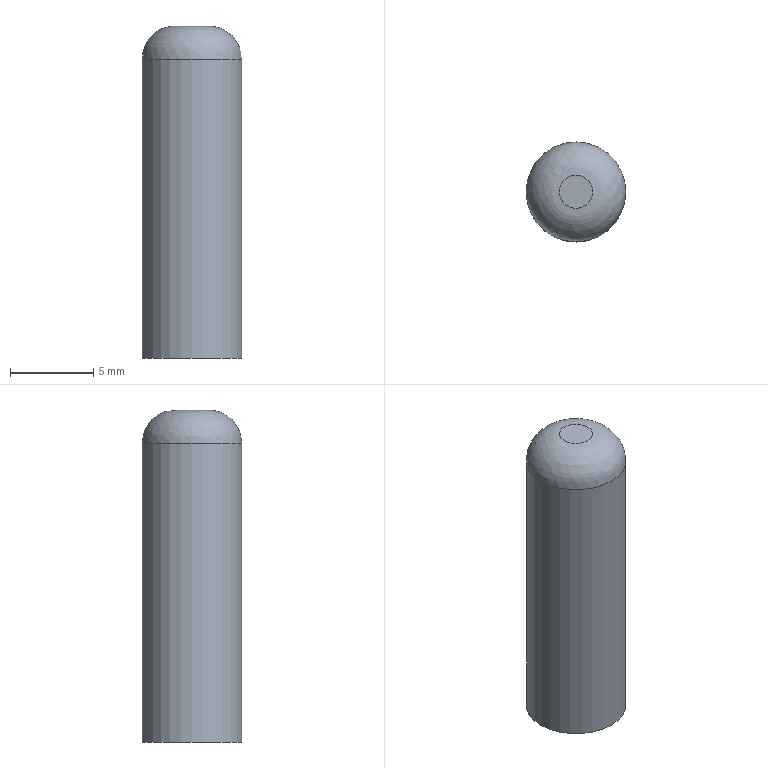Part | STEP file | SynoNew-0304-062 | 1 solid | 4 faces | box 6 x 6 x 20 mm | volume 551.703 mm3 | plane 2 | spline 1 | cylinder 1 | commonest cylinder face diameters 6 x1
STEP:
#1=CARTESIAN_POINT('',(1.,0.,20.));
#2=VERTEX_POINT('',#1);
#3=CARTESIAN_POINT('',(-1.,0.,20.));
#4=VERTEX_POINT('',#3);
#5=CARTESIAN_POINT('',(0.,0.,20.));
#6=DIRECTION('',(0.,0.,-1.));
#7=DIRECTION('',(-1.,0.,0.));
#8=AXIS2_PLACEMENT_3D('',#5,#6,#7);
#9=CIRCLE('',#8,1.);
#10=EDGE_CURVE('',#2,#4,#9,.T.);
#11=ORIENTED_EDGE('',*,*,#10,.T.);
#12=CARTESIAN_POINT('',(-3.,0.,18.));
#13=VERTEX_POINT('',#12);
#14=CARTESIAN_POINT('',(-1.,0.,18.));
#15=DIRECTION('',(0.,-1.,0.));
#16=DIRECTION('',(-1.,0.,0.));
#17=AXIS2_PLACEMENT_3D('',#14,#15,#16);
#18=CIRCLE('',#17,2.);
#19=EDGE_CURVE('',#4,#13,#18,.T.);
#20=ORIENTED_EDGE('',*,*,#19,.T.);
#21=CARTESIAN_POINT('',(3.,0.,18.));
#22=VERTEX_POINT('',#21);
#23=CARTESIAN_POINT('',(0.,0.,18.));
#24=DIRECTION('',(0.,0.,1.));
#25=DIRECTION('',(-1.,0.,0.));
#26=AXIS2_PLACEMENT_3D('',#23,#24,#25);
#27=CIRCLE('',#26,3.);
#28=EDGE_CURVE('',#13,#22,#27,.T.);
#29=ORIENTED_EDGE('',*,*,#28,.T.);
#30=CARTESIAN_POINT('',(0.,0.,18.));
#31=DIRECTION('',(0.,0.,1.));
#32=DIRECTION('',(-1.,0.,0.));
#33=AXIS2_PLACEMENT_3D('',#30,#31,#32);
#34=CIRCLE('',#33,3.);
#35=EDGE_CURVE('',#22,#13,#34,.T.);
#36=ORIENTED_EDGE('',*,*,#35,.T.);
#37=ORIENTED_EDGE('',*,*,#19,.F.);
#38=CARTESIAN_POINT('',(0.,0.,20.));
#39=DIRECTION('',(0.,0.,-1.));
#40=DIRECTION('',(-1.,0.,0.));
#41=AXIS2_PLACEMENT_3D('',#38,#39,#40);
#42=CIRCLE('',#41,1.);
#43=EDGE_CURVE('',#4,#2,#42,.T.);
#44=ORIENTED_EDGE('',*,*,#43,.T.);
#45=EDGE_LOOP('',(#11,#20,#29,#36,#37,#44));
#46=FACE_OUTER_BOUND('',#45,.T.);
#47=CARTESIAN_POINT('',(-3.,0.,18.));
#48=CARTESIAN_POINT('',(-3.,-3.,18.));
#49=CARTESIAN_POINT('',(0.,-3.,18.));
#50=CARTESIAN_POINT('',(3.,-3.,18.));
#51=CARTESIAN_POINT('',(3.,0.,18.));
#52=CARTESIAN_POINT('',(3.,3.,18.));
#53=CARTESIAN_POINT('',(0.,3.,18.));
#54=CARTESIAN_POINT('',(-3.,3.,18.));
#55=CARTESIAN_POINT('',(-3.,0.,18.));
#56=CARTESIAN_POINT('',(-3.,0.,20.));
#57=CARTESIAN_POINT('',(-3.,-3.,20.));
#58=CARTESIAN_POINT('',(0.,-3.,20.));
#59=CARTESIAN_POINT('',(3.,-3.,20.));
#60=CARTESIAN_POINT('',(3.,0.,20.));
#61=CARTESIAN_POINT('',(3.,3.,20.));
#62=CARTESIAN_POINT('',(0.,3.,20.));
#63=CARTESIAN_POINT('',(-3.,3.,20.));
#64=CARTESIAN_POINT('',(-3.,0.,20.));
#65=CARTESIAN_POINT('',(-1.,0.,20.));
#66=CARTESIAN_POINT('',(-1.,-1.,20.));
#67=CARTESIAN_POINT('',(0.,-1.,20.));
#68=CARTESIAN_POINT('',(1.,-1.,20.));
#69=CARTESIAN_POINT('',(1.,0.,20.));
#70=CARTESIAN_POINT('',(1.,1.,20.));
#71=CARTESIAN_POINT('',(0.,1.,20.));
#72=CARTESIAN_POINT('',(-1.,1.,20.));
#73=CARTESIAN_POINT('',(-1.,0.,20.));
#74=(BOUNDED_SURFACE()B_SPLINE_SURFACE(2,2,((#47,#48,#49,#50,#51,#52,#53,#54,#55),(#56,#57,#58,#59,#60,#61,#62,#63,#64),(#65,#66,#67,#68,#69,#70,#71,#72,#73)),.UNSPECIFIED.,.F.,.T.,.F.)B_SPLINE_SURFACE_WITH_KNOTS((3,3),(3,2,2,2,3),(0.,1.571),(-3.142,-1.571,0.,1.571,3.142),.UNSPECIFIED.)GEOMETRIC_REPRESENTATION_ITEM()RATIONAL_B_SPLINE_SURFACE(((1.,0.7071,1.,0.7071,1.,0.7071,1.,0.7071,1.),(0.7071,0.5,0.7071,0.5,0.7071,0.5,0.7071,0.5,0.7071),(1.,0.7071,1.,0.7071,1.,0.7071,1.,0.7071,1.)))REPRESENTATION_ITEM('')SURFACE());
#75=ADVANCED_FACE('',(#46),#74,.F.);
#76=ORIENTED_EDGE('',*,*,#35,.F.);
#77=ORIENTED_EDGE('',*,*,#28,.F.);
#78=CARTESIAN_POINT('',(-3.,0.,0.));
#79=VERTEX_POINT('',#78);
#80=CARTESIAN_POINT('',(-3.,0.,0.));
#81=DIRECTION('',(0.,0.,-1.));
#82=VECTOR('',#81,3.);
#83=LINE('',#80,#82);
#84=EDGE_CURVE('',#13,#79,#83,.T.);
#85=ORIENTED_EDGE('',*,*,#84,.T.);
#86=CARTESIAN_POINT('',(3.,0.,0.));
#87=VERTEX_POINT('',#86);
#88=CARTESIAN_POINT('',(0.,0.,0.));
#89=DIRECTION('',(0.,0.,1.));
#90=DIRECTION('',(1.,0.,0.));
#91=AXIS2_PLACEMENT_3D('',#88,#89,#90);
#92=CIRCLE('',#91,3.);
#93=EDGE_CURVE('',#79,#87,#92,.T.);
#94=ORIENTED_EDGE('',*,*,#93,.T.);
#95=CARTESIAN_POINT('',(0.,0.,0.));
#96=DIRECTION('',(0.,0.,1.));
#97=DIRECTION('',(1.,0.,0.));
#98=AXIS2_PLACEMENT_3D('',#95,#96,#97);
#99=CIRCLE('',#98,3.);
#100=EDGE_CURVE('',#87,#79,#99,.T.);
#101=ORIENTED_EDGE('',*,*,#100,.T.);
#102=ORIENTED_EDGE('',*,*,#84,.F.);
#103=EDGE_LOOP('',(#76,#77,#85,#94,#101,#102));
#104=FACE_OUTER_BOUND('',#103,.T.);
#105=CARTESIAN_POINT('',(0.,0.,0.));
#106=DIRECTION('',(0.,0.,1.));
#107=DIRECTION('',(1.,0.,0.));
#108=AXIS2_PLACEMENT_3D('',#105,#106,#107);
#109=CYLINDRICAL_SURFACE('',#108,3.);
#110=ADVANCED_FACE('',(#104),#109,.T.);
#111=ORIENTED_EDGE('',*,*,#10,.F.);
#112=ORIENTED_EDGE('',*,*,#43,.F.);
#113=EDGE_LOOP('',(#111,#112));
#114=FACE_OUTER_BOUND('',#113,.T.);
#115=CARTESIAN_POINT('',(0.,0.,20.));
#116=DIRECTION('',(0.,0.,1.));
#117=DIRECTION('',(1.,0.,0.));
#118=AXIS2_PLACEMENT_3D('',#115,#116,#117);
#119=PLANE('',#118);
#120=ADVANCED_FACE('',(#114),#119,.T.);
#121=ORIENTED_EDGE('',*,*,#100,.F.);
#122=ORIENTED_EDGE('',*,*,#93,.F.);
#123=EDGE_LOOP('',(#121,#122));
#124=FACE_OUTER_BOUND('',#123,.T.);
#125=CARTESIAN_POINT('',(0.,0.,0.));
#126=DIRECTION('',(0.,0.,1.));
#127=DIRECTION('',(1.,0.,0.));
#128=AXIS2_PLACEMENT_3D('',#125,#126,#127);
#129=PLANE('',#128);
#130=ADVANCED_FACE('',(#124),#129,.F.);
#131=CLOSED_SHELL('',(#75,#110,#120,#130));
#132=MANIFOLD_SOLID_BREP('',#131);
#133=(LENGTH_UNIT()NAMED_UNIT(*)SI_UNIT(.MILLI.,.METRE.));
#134=UNCERTAINTY_MEASURE_WITH_UNIT(LENGTH_MEASURE(0.01),#133,'','');
#135=(NAMED_UNIT(*)PLANE_ANGLE_UNIT()SI_UNIT($,.RADIAN.));
#136=(NAMED_UNIT(*)SI_UNIT($,.STERADIAN.)SOLID_ANGLE_UNIT());
#137=(GEOMETRIC_REPRESENTATION_CONTEXT(3)GLOBAL_UNCERTAINTY_ASSIGNED_CONTEXT((#134))GLOBAL_UNIT_ASSIGNED_CONTEXT((#133,#135,#136))REPRESENTATION_CONTEXT('',''));
#138=ADVANCED_BREP_SHAPE_REPRESENTATION('',(#132),#137);